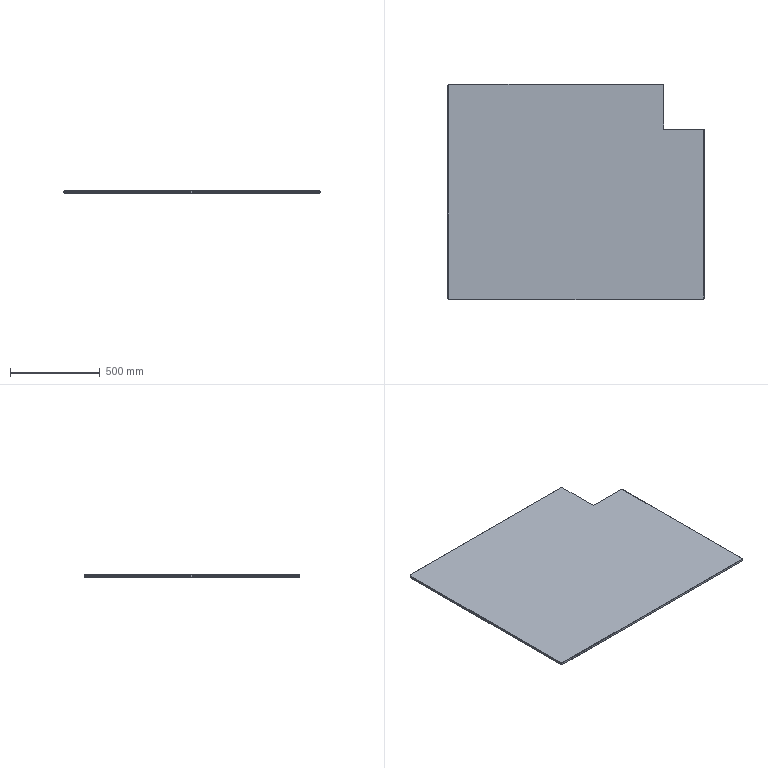Part | STEP file | 1200x1425x13 aluminium plateC-1.STEP | 1 solid | 25 faces | box 1425 x 1200 x 13 mm | volume 21493737 mm3 | plane 16 | cone 6 | cylinder 3 | commonest cylinder face diameters 20 x3
STEP:
#1=CARTESIAN_POINT('',(712.5,350.2,1.));
#2=VERTEX_POINT('',#1);
#3=CARTESIAN_POINT('',(711.5,350.2,0.));
#4=VERTEX_POINT('',#3);
#5=CARTESIAN_POINT('',(712.5,350.2,1.));
#6=DIRECTION('',(-0.7071,0.,-0.7071));
#7=VECTOR('',#6,1000.);
#8=LINE('',#5,#7);
#9=EDGE_CURVE('',#2,#4,#8,.T.);
#10=ORIENTED_EDGE('',*,*,#9,.T.);
#11=CARTESIAN_POINT('',(487.5,350.2,0.));
#12=VERTEX_POINT('',#11);
#13=CARTESIAN_POINT('',(712.5,350.2,0.));
#14=DIRECTION('',(-1.,0.,0.));
#15=VECTOR('',#14,1000.);
#16=LINE('',#13,#15);
#17=EDGE_CURVE('',#4,#12,#16,.T.);
#18=ORIENTED_EDGE('',*,*,#17,.T.);
#19=CARTESIAN_POINT('',(487.5,350.2,13.));
#20=VERTEX_POINT('',#19);
#21=CARTESIAN_POINT('',(487.5,350.2,13.));
#22=DIRECTION('',(0.,0.,-1.));
#23=VECTOR('',#22,1000.);
#24=LINE('',#21,#23);
#25=EDGE_CURVE('',#20,#12,#24,.T.);
#26=ORIENTED_EDGE('',*,*,#25,.F.);
#27=CARTESIAN_POINT('',(711.5,350.2,13.));
#28=VERTEX_POINT('',#27);
#29=CARTESIAN_POINT('',(712.5,350.2,13.));
#30=DIRECTION('',(-1.,0.,0.));
#31=VECTOR('',#30,1000.);
#32=LINE('',#29,#31);
#33=EDGE_CURVE('',#28,#20,#32,.T.);
#34=ORIENTED_EDGE('',*,*,#33,.F.);
#35=CARTESIAN_POINT('',(712.5,350.2,12.));
#36=VERTEX_POINT('',#35);
#37=CARTESIAN_POINT('',(711.5,350.2,13.));
#38=DIRECTION('',(0.7071,0.,-0.7071));
#39=VECTOR('',#38,1000.);
#40=LINE('',#37,#39);
#41=EDGE_CURVE('',#28,#36,#40,.T.);
#42=ORIENTED_EDGE('',*,*,#41,.T.);
#43=CARTESIAN_POINT('',(712.5,350.2,13.));
#44=DIRECTION('',(0.,0.,-1.));
#45=VECTOR('',#44,1000.);
#46=LINE('',#43,#45);
#47=EDGE_CURVE('',#36,#2,#46,.T.);
#48=ORIENTED_EDGE('',*,*,#47,.T.);
#49=EDGE_LOOP('',(#10,#18,#26,#34,#42,#48));
#50=FACE_OUTER_BOUND('',#49,.T.);
#51=CARTESIAN_POINT('',(712.5,350.2,13.));
#52=DIRECTION('',(0.,-1.,0.));
#53=DIRECTION('',(0.,0.,-1.));
#54=AXIS2_PLACEMENT_3D('',#51,#52,#53);
#55=PLANE('',#54);
#56=ADVANCED_FACE('',(#50),#55,.F.);
#57=CARTESIAN_POINT('',(487.5,599.,0.));
#58=VERTEX_POINT('',#57);
#59=CARTESIAN_POINT('',(487.5,600.,1.));
#60=VERTEX_POINT('',#59);
#61=CARTESIAN_POINT('',(487.5,600.,1.));
#62=DIRECTION('',(0.,0.7071,0.7071));
#63=VECTOR('',#62,1000.);
#64=LINE('',#61,#63);
#65=EDGE_CURVE('',#58,#60,#64,.T.);
#66=ORIENTED_EDGE('',*,*,#65,.T.);
#67=CARTESIAN_POINT('',(487.5,600.,12.));
#68=VERTEX_POINT('',#67);
#69=CARTESIAN_POINT('',(487.5,600.,13.));
#70=DIRECTION('',(0.,0.,-1.));
#71=VECTOR('',#70,1000.);
#72=LINE('',#69,#71);
#73=EDGE_CURVE('',#68,#60,#72,.T.);
#74=ORIENTED_EDGE('',*,*,#73,.F.);
#75=CARTESIAN_POINT('',(487.5,599.,13.));
#76=VERTEX_POINT('',#75);
#77=CARTESIAN_POINT('',(487.5,599.,13.));
#78=DIRECTION('',(0.,-0.7071,0.7071));
#79=VECTOR('',#78,1000.);
#80=LINE('',#77,#79);
#81=EDGE_CURVE('',#68,#76,#80,.T.);
#82=ORIENTED_EDGE('',*,*,#81,.T.);
#83=CARTESIAN_POINT('',(487.5,600.,13.));
#84=DIRECTION('',(0.,1.,0.));
#85=VECTOR('',#84,1000.);
#86=LINE('',#83,#85);
#87=EDGE_CURVE('',#20,#76,#86,.T.);
#88=ORIENTED_EDGE('',*,*,#87,.F.);
#89=ORIENTED_EDGE('',*,*,#25,.T.);
#90=CARTESIAN_POINT('',(487.5,600.,0.));
#91=DIRECTION('',(0.,1.,0.));
#92=VECTOR('',#91,1000.);
#93=LINE('',#90,#92);
#94=EDGE_CURVE('',#12,#58,#93,.T.);
#95=ORIENTED_EDGE('',*,*,#94,.T.);
#96=EDGE_LOOP('',(#66,#74,#82,#88,#89,#95));
#97=FACE_OUTER_BOUND('',#96,.T.);
#98=CARTESIAN_POINT('',(487.5,600.,13.));
#99=DIRECTION('',(-1.,0.,0.));
#100=DIRECTION('',(0.,0.,1.));
#101=AXIS2_PLACEMENT_3D('',#98,#99,#100);
#102=PLANE('',#101);
#103=ADVANCED_FACE('',(#97),#102,.F.);
#104=CARTESIAN_POINT('',(-702.5,599.,13.));
#105=VERTEX_POINT('',#104);
#106=CARTESIAN_POINT('',(-702.5,600.,12.));
#107=VERTEX_POINT('',#106);
#108=CARTESIAN_POINT('',(-702.5,599.,13.));
#109=DIRECTION('',(0.,0.7071,-0.7071));
#110=VECTOR('',#109,1000.);
#111=LINE('',#108,#110);
#112=EDGE_CURVE('',#105,#107,#111,.T.);
#113=ORIENTED_EDGE('',*,*,#112,.T.);
#114=CARTESIAN_POINT('',(-712.5,590.,12.));
#115=VERTEX_POINT('',#114);
#116=CARTESIAN_POINT('',(-702.5,590.,12.));
#117=DIRECTION('',(0.,0.,-1.));
#118=DIRECTION('',(1.,0.,0.));
#119=AXIS2_PLACEMENT_3D('',#116,#117,#118);
#120=CIRCLE('',#119,10.);
#121=EDGE_CURVE('',#115,#107,#120,.T.);
#122=ORIENTED_EDGE('',*,*,#121,.F.);
#123=CARTESIAN_POINT('',(-711.5,590.,13.));
#124=VERTEX_POINT('',#123);
#125=CARTESIAN_POINT('',(-712.5,590.,12.));
#126=DIRECTION('',(0.7071,0.,0.7071));
#127=VECTOR('',#126,1000.);
#128=LINE('',#125,#127);
#129=EDGE_CURVE('',#115,#124,#128,.T.);
#130=ORIENTED_EDGE('',*,*,#129,.T.);
#131=CARTESIAN_POINT('',(-702.5,590.,13.));
#132=DIRECTION('',(0.,0.,1.));
#133=DIRECTION('',(1.,0.,0.));
#134=AXIS2_PLACEMENT_3D('',#131,#132,#133);
#135=CIRCLE('',#134,9.);
#136=EDGE_CURVE('',#105,#124,#135,.T.);
#137=ORIENTED_EDGE('',*,*,#136,.F.);
#138=EDGE_LOOP('',(#113,#122,#130,#137));
#139=FACE_OUTER_BOUND('',#138,.T.);
#140=CARTESIAN_POINT('',(-702.5,590.,13.));
#141=DIRECTION('',(0.,0.,-1.));
#142=DIRECTION('',(-1.,0.,0.));
#143=AXIS2_PLACEMENT_3D('',#140,#141,#142);
#144=CONICAL_SURFACE('',#143,9.,0.7854);
#145=ADVANCED_FACE('',(#139),#144,.T.);
#146=CARTESIAN_POINT('',(-712.5,-590.,12.));
#147=VERTEX_POINT('',#146);
#148=CARTESIAN_POINT('',(-711.5,-590.,13.));
#149=VERTEX_POINT('',#148);
#150=CARTESIAN_POINT('',(-712.5,-590.,12.));
#151=DIRECTION('',(0.7071,0.,0.7071));
#152=VECTOR('',#151,1000.);
#153=LINE('',#150,#152);
#154=EDGE_CURVE('',#147,#149,#153,.T.);
#155=ORIENTED_EDGE('',*,*,#154,.T.);
#156=CARTESIAN_POINT('',(-711.5,-590.,13.));
#157=DIRECTION('',(0.,-1.,0.));
#158=VECTOR('',#157,1000.);
#159=LINE('',#156,#158);
#160=EDGE_CURVE('',#124,#149,#159,.T.);
#161=ORIENTED_EDGE('',*,*,#160,.F.);
#162=ORIENTED_EDGE('',*,*,#129,.F.);
#163=CARTESIAN_POINT('',(-712.5,590.,12.));
#164=DIRECTION('',(0.,1.,0.));
#165=VECTOR('',#164,1000.);
#166=LINE('',#163,#165);
#167=EDGE_CURVE('',#147,#115,#166,.T.);
#168=ORIENTED_EDGE('',*,*,#167,.F.);
#169=EDGE_LOOP('',(#155,#161,#162,#168));
#170=FACE_OUTER_BOUND('',#169,.T.);
#171=CARTESIAN_POINT('',(-711.5,0.,13.));
#172=DIRECTION('',(-0.7071,0.,0.7071));
#173=DIRECTION('',(0.,1.,0.));
#174=AXIS2_PLACEMENT_3D('',#171,#172,#173);
#175=PLANE('',#174);
#176=ADVANCED_FACE('',(#170),#175,.T.);
#177=ORIENTED_EDGE('',*,*,#81,.F.);
#178=CARTESIAN_POINT('',(702.5,600.,12.));
#179=DIRECTION('',(1.,0.,0.));
#180=VECTOR('',#179,1000.);
#181=LINE('',#178,#180);
#182=EDGE_CURVE('',#107,#68,#181,.T.);
#183=ORIENTED_EDGE('',*,*,#182,.F.);
#184=ORIENTED_EDGE('',*,*,#112,.F.);
#185=CARTESIAN_POINT('',(-702.5,599.,13.));
#186=DIRECTION('',(-1.,0.,0.));
#187=VECTOR('',#186,1000.);
#188=LINE('',#185,#187);
#189=EDGE_CURVE('',#76,#105,#188,.T.);
#190=ORIENTED_EDGE('',*,*,#189,.F.);
#191=EDGE_LOOP('',(#177,#183,#184,#190));
#192=FACE_OUTER_BOUND('',#191,.T.);
#193=CARTESIAN_POINT('',(0.,599.,13.));
#194=DIRECTION('',(0.,0.7071,0.7071));
#195=DIRECTION('',(1.,0.,0.));
#196=AXIS2_PLACEMENT_3D('',#193,#194,#195);
#197=PLANE('',#196);
#198=ADVANCED_FACE('',(#192),#197,.T.);
#199=CARTESIAN_POINT('',(-702.5,-600.,12.));
#200=VERTEX_POINT('',#199);
#201=CARTESIAN_POINT('',(-702.5,-599.,13.));
#202=VERTEX_POINT('',#201);
#203=CARTESIAN_POINT('',(-702.5,-600.,12.));
#204=DIRECTION('',(0.,0.7071,0.7071));
#205=VECTOR('',#204,1000.);
#206=LINE('',#203,#205);
#207=EDGE_CURVE('',#200,#202,#206,.T.);
#208=ORIENTED_EDGE('',*,*,#207,.T.);
#209=CARTESIAN_POINT('',(-702.5,-590.,13.));
#210=DIRECTION('',(0.,0.,1.));
#211=DIRECTION('',(1.,0.,0.));
#212=AXIS2_PLACEMENT_3D('',#209,#210,#211);
#213=CIRCLE('',#212,9.);
#214=EDGE_CURVE('',#149,#202,#213,.T.);
#215=ORIENTED_EDGE('',*,*,#214,.F.);
#216=ORIENTED_EDGE('',*,*,#154,.F.);
#217=CARTESIAN_POINT('',(-702.5,-590.,12.));
#218=DIRECTION('',(0.,0.,-1.));
#219=DIRECTION('',(1.,0.,0.));
#220=AXIS2_PLACEMENT_3D('',#217,#218,#219);
#221=CIRCLE('',#220,10.);
#222=EDGE_CURVE('',#200,#147,#221,.T.);
#223=ORIENTED_EDGE('',*,*,#222,.F.);
#224=EDGE_LOOP('',(#208,#215,#216,#223));
#225=FACE_OUTER_BOUND('',#224,.T.);
#226=CARTESIAN_POINT('',(-702.5,-590.,13.));
#227=DIRECTION('',(0.,0.,-1.));
#228=DIRECTION('',(-1.,0.,0.));
#229=AXIS2_PLACEMENT_3D('',#226,#227,#228);
#230=CONICAL_SURFACE('',#229,9.,0.7854);
#231=ADVANCED_FACE('',(#225),#230,.T.);
#232=CARTESIAN_POINT('',(702.5,-600.,12.));
#233=VERTEX_POINT('',#232);
#234=CARTESIAN_POINT('',(702.5,-599.,13.));
#235=VERTEX_POINT('',#234);
#236=CARTESIAN_POINT('',(702.5,-600.,12.));
#237=DIRECTION('',(0.,0.7071,0.7071));
#238=VECTOR('',#237,1000.);
#239=LINE('',#236,#238);
#240=EDGE_CURVE('',#233,#235,#239,.T.);
#241=ORIENTED_EDGE('',*,*,#240,.T.);
#242=CARTESIAN_POINT('',(702.5,-599.,13.));
#243=DIRECTION('',(1.,0.,0.));
#244=VECTOR('',#243,1000.);
#245=LINE('',#242,#244);
#246=EDGE_CURVE('',#202,#235,#245,.T.);
#247=ORIENTED_EDGE('',*,*,#246,.F.);
#248=ORIENTED_EDGE('',*,*,#207,.F.);
#249=CARTESIAN_POINT('',(-702.5,-600.,12.));
#250=DIRECTION('',(-1.,0.,0.));
#251=VECTOR('',#250,1000.);
#252=LINE('',#249,#251);
#253=EDGE_CURVE('',#233,#200,#252,.T.);
#254=ORIENTED_EDGE('',*,*,#253,.F.);
#255=EDGE_LOOP('',(#241,#247,#248,#254));
#256=FACE_OUTER_BOUND('',#255,.T.);
#257=CARTESIAN_POINT('',(0.,-599.,13.));
#258=DIRECTION('',(0.,-0.7071,0.7071));
#259=DIRECTION('',(-1.,0.,0.));
#260=AXIS2_PLACEMENT_3D('',#257,#258,#259);
#261=PLANE('',#260);
#262=ADVANCED_FACE('',(#256),#261,.T.);
#263=ORIENTED_EDGE('',*,*,#41,.F.);
#264=CARTESIAN_POINT('',(711.5,-590.,13.));
#265=VERTEX_POINT('',#264);
#266=CARTESIAN_POINT('',(711.5,590.,13.));
#267=DIRECTION('',(0.,1.,0.));
#268=VECTOR('',#267,1000.);
#269=LINE('',#266,#268);
#270=EDGE_CURVE('',#265,#28,#269,.T.);
#271=ORIENTED_EDGE('',*,*,#270,.F.);
#272=CARTESIAN_POINT('',(712.5,-590.,12.));
#273=VERTEX_POINT('',#272);
#274=CARTESIAN_POINT('',(711.5,-590.,13.));
#275=DIRECTION('',(0.7071,0.,-0.7071));
#276=VECTOR('',#275,1000.);
#277=LINE('',#274,#276);
#278=EDGE_CURVE('',#265,#273,#277,.T.);
#279=ORIENTED_EDGE('',*,*,#278,.T.);
#280=CARTESIAN_POINT('',(712.5,-590.,12.));
#281=DIRECTION('',(0.,-1.,0.));
#282=VECTOR('',#281,1000.);
#283=LINE('',#280,#282);
#284=EDGE_CURVE('',#36,#273,#283,.T.);
#285=ORIENTED_EDGE('',*,*,#284,.F.);
#286=EDGE_LOOP('',(#263,#271,#279,#285));
#287=FACE_OUTER_BOUND('',#286,.T.);
#288=CARTESIAN_POINT('',(711.5,0.,13.));
#289=DIRECTION('',(0.7071,0.,0.7071));
#290=DIRECTION('',(0.,-1.,0.));
#291=AXIS2_PLACEMENT_3D('',#288,#289,#290);
#292=PLANE('',#291);
#293=ADVANCED_FACE('',(#287),#292,.T.);
#294=ORIENTED_EDGE('',*,*,#240,.F.);
#295=CARTESIAN_POINT('',(702.5,-590.,12.));
#296=DIRECTION('',(0.,0.,-1.));
#297=DIRECTION('',(1.,0.,0.));
#298=AXIS2_PLACEMENT_3D('',#295,#296,#297);
#299=CIRCLE('',#298,10.);
#300=EDGE_CURVE('',#273,#233,#299,.T.);
#301=ORIENTED_EDGE('',*,*,#300,.F.);
#302=ORIENTED_EDGE('',*,*,#278,.F.);
#303=CARTESIAN_POINT('',(702.5,-590.,13.));
#304=DIRECTION('',(0.,0.,1.));
#305=DIRECTION('',(1.,0.,0.));
#306=AXIS2_PLACEMENT_3D('',#303,#304,#305);
#307=CIRCLE('',#306,9.);
#308=EDGE_CURVE('',#235,#265,#307,.T.);
#309=ORIENTED_EDGE('',*,*,#308,.F.);
#310=EDGE_LOOP('',(#294,#301,#302,#309));
#311=FACE_OUTER_BOUND('',#310,.T.);
#312=CARTESIAN_POINT('',(702.5,-590.,13.));
#313=DIRECTION('',(0.,0.,-1.));
#314=DIRECTION('',(-1.,0.,0.));
#315=AXIS2_PLACEMENT_3D('',#312,#313,#314);
#316=CONICAL_SURFACE('',#315,9.,0.7854);
#317=ADVANCED_FACE('',(#311),#316,.T.);
#318=CARTESIAN_POINT('',(711.5,-590.,0.));
#319=VERTEX_POINT('',#318);
#320=CARTESIAN_POINT('',(712.5,-590.,1.));
#321=VERTEX_POINT('',#320);
#322=CARTESIAN_POINT('',(711.5,-590.,0.));
#323=DIRECTION('',(0.7071,0.,0.7071));
#324=VECTOR('',#323,1000.);
#325=LINE('',#322,#324);
#326=EDGE_CURVE('',#319,#321,#325,.T.);
#327=ORIENTED_EDGE('',*,*,#326,.T.);
#328=CARTESIAN_POINT('',(702.5,-600.,1.));
#329=VERTEX_POINT('',#328);
#330=CARTESIAN_POINT('',(702.5,-590.,1.));
#331=DIRECTION('',(0.,0.,1.));
#332=DIRECTION('',(1.,0.,0.));
#333=AXIS2_PLACEMENT_3D('',#330,#331,#332);
#334=CIRCLE('',#333,10.);
#335=EDGE_CURVE('',#329,#321,#334,.T.);
#336=ORIENTED_EDGE('',*,*,#335,.F.);
#337=CARTESIAN_POINT('',(702.5,-599.,0.));
#338=VERTEX_POINT('',#337);
#339=CARTESIAN_POINT('',(702.5,-600.,1.));
#340=DIRECTION('',(0.,0.7071,-0.7071));
#341=VECTOR('',#340,1000.);
#342=LINE('',#339,#341);
#343=EDGE_CURVE('',#329,#338,#342,.T.);
#344=ORIENTED_EDGE('',*,*,#343,.T.);
#345=CARTESIAN_POINT('',(702.5,-590.,0.));
#346=DIRECTION('',(0.,0.,-1.));
#347=DIRECTION('',(1.,0.,0.));
#348=AXIS2_PLACEMENT_3D('',#345,#346,#347);
#349=CIRCLE('',#348,9.);
#350=EDGE_CURVE('',#319,#338,#349,.T.);
#351=ORIENTED_EDGE('',*,*,#350,.F.);
#352=EDGE_LOOP('',(#327,#336,#344,#351));
#353=FACE_OUTER_BOUND('',#352,.T.);
#354=CARTESIAN_POINT('',(702.5,-590.,0.));
#355=DIRECTION('',(0.,0.,1.));
#356=DIRECTION('',(1.,0.,0.));
#357=AXIS2_PLACEMENT_3D('',#354,#355,#356);
#358=CONICAL_SURFACE('',#357,9.,0.7854);
#359=ADVANCED_FACE('',(#353),#358,.T.);
#360=CARTESIAN_POINT('',(-702.5,-600.,1.));
#361=VERTEX_POINT('',#360);
#362=CARTESIAN_POINT('',(-702.5,-599.,0.));
#363=VERTEX_POINT('',#362);
#364=CARTESIAN_POINT('',(-702.5,-600.,1.));
#365=DIRECTION('',(0.,0.7071,-0.7071));
#366=VECTOR('',#365,1000.);
#367=LINE('',#364,#366);
#368=EDGE_CURVE('',#361,#363,#367,.T.);
#369=ORIENTED_EDGE('',*,*,#368,.T.);
#370=CARTESIAN_POINT('',(0.,-599.,0.));
#371=DIRECTION('',(-1.,0.,0.));
#372=VECTOR('',#371,1000.);
#373=LINE('',#370,#372);
#374=EDGE_CURVE('',#338,#363,#373,.T.);
#375=ORIENTED_EDGE('',*,*,#374,.F.);
#376=ORIENTED_EDGE('',*,*,#343,.F.);
#377=CARTESIAN_POINT('',(-712.5,-600.,1.));
#378=DIRECTION('',(1.,0.,0.));
#379=VECTOR('',#378,1000.);
#380=LINE('',#377,#379);
#381=EDGE_CURVE('',#361,#329,#380,.T.);
#382=ORIENTED_EDGE('',*,*,#381,.F.);
#383=EDGE_LOOP('',(#369,#375,#376,#382));
#384=FACE_OUTER_BOUND('',#383,.T.);
#385=CARTESIAN_POINT('',(-712.5,-600.,1.));
#386=DIRECTION('',(0.,0.7071,0.7071));
#387=DIRECTION('',(1.,0.,0.));
#388=AXIS2_PLACEMENT_3D('',#385,#386,#387);
#389=PLANE('',#388);
#390=ADVANCED_FACE('',(#384),#389,.F.);
#391=ORIENTED_EDGE('',*,*,#9,.F.);
#392=CARTESIAN_POINT('',(712.5,600.,1.));
#393=DIRECTION('',(0.,1.,0.));
#394=VECTOR('',#393,1000.);
#395=LINE('',#392,#394);
#396=EDGE_CURVE('',#321,#2,#395,.T.);
#397=ORIENTED_EDGE('',*,*,#396,.F.);
#398=ORIENTED_EDGE('',*,*,#326,.F.);
#399=CARTESIAN_POINT('',(711.5,0.,0.));
#400=DIRECTION('',(0.,-1.,0.));
#401=VECTOR('',#400,1000.);
#402=LINE('',#399,#401);
#403=EDGE_CURVE('',#4,#319,#402,.T.);
#404=ORIENTED_EDGE('',*,*,#403,.F.);
#405=EDGE_LOOP('',(#391,#397,#398,#404));
#406=FACE_OUTER_BOUND('',#405,.T.);
#407=CARTESIAN_POINT('',(712.5,600.,1.));
#408=DIRECTION('',(-0.7071,0.,0.7071));
#409=DIRECTION('',(0.,1.,0.));
#410=AXIS2_PLACEMENT_3D('',#407,#408,#409);
#411=PLANE('',#410);
#412=ADVANCED_FACE('',(#406),#411,.F.);
#413=CARTESIAN_POINT('',(-712.5,-590.,1.));
#414=VERTEX_POINT('',#413);
#415=CARTESIAN_POINT('',(-711.5,-590.,0.));
#416=VERTEX_POINT('',#415);
#417=CARTESIAN_POINT('',(-712.5,-590.,1.));
#418=DIRECTION('',(0.7071,0.,-0.7071));
#419=VECTOR('',#418,1000.);
#420=LINE('',#417,#419);
#421=EDGE_CURVE('',#414,#416,#420,.T.);
#422=ORIENTED_EDGE('',*,*,#421,.T.);
#423=CARTESIAN_POINT('',(-702.5,-590.,0.));
#424=DIRECTION('',(0.,0.,-1.));
#425=DIRECTION('',(1.,0.,0.));
#426=AXIS2_PLACEMENT_3D('',#423,#424,#425);
#427=CIRCLE('',#426,9.);
#428=EDGE_CURVE('',#363,#416,#427,.T.);
#429=ORIENTED_EDGE('',*,*,#428,.F.);
#430=ORIENTED_EDGE('',*,*,#368,.F.);
#431=CARTESIAN_POINT('',(-702.5,-590.,1.));
#432=DIRECTION('',(0.,0.,1.));
#433=DIRECTION('',(1.,0.,0.));
#434=AXIS2_PLACEMENT_3D('',#431,#432,#433);
#435=CIRCLE('',#434,10.);
#436=EDGE_CURVE('',#414,#361,#435,.T.);
#437=ORIENTED_EDGE('',*,*,#436,.F.);
#438=EDGE_LOOP('',(#422,#429,#430,#437));
#439=FACE_OUTER_BOUND('',#438,.T.);
#440=CARTESIAN_POINT('',(-702.5,-590.,0.));
#441=DIRECTION('',(0.,0.,1.));
#442=DIRECTION('',(1.,0.,0.));
#443=AXIS2_PLACEMENT_3D('',#440,#441,#442);
#444=CONICAL_SURFACE('',#443,9.,0.7854);
#445=ADVANCED_FACE('',(#439),#444,.T.);
#446=CARTESIAN_POINT('',(-712.5,590.,1.));
#447=VERTEX_POINT('',#446);
#448=CARTESIAN_POINT('',(-711.5,590.,0.));
#449=VERTEX_POINT('',#448);
#450=CARTESIAN_POINT('',(-712.5,590.,1.));
#451=DIRECTION('',(0.7071,0.,-0.7071));
#452=VECTOR('',#451,1000.);
#453=LINE('',#450,#452);
#454=EDGE_CURVE('',#447,#449,#453,.T.);
#455=ORIENTED_EDGE('',*,*,#454,.T.);
#456=CARTESIAN_POINT('',(-711.5,0.,0.));
#457=DIRECTION('',(0.,1.,0.));
#458=VECTOR('',#457,1000.);
#459=LINE('',#456,#458);
#460=EDGE_CURVE('',#416,#449,#459,.T.);
#461=ORIENTED_EDGE('',*,*,#460,.F.);
#462=ORIENTED_EDGE('',*,*,#421,.F.);
#463=CARTESIAN_POINT('',(-712.5,600.,1.));
#464=DIRECTION('',(0.,-1.,0.));
#465=VECTOR('',#464,1000.);
#466=LINE('',#463,#465);
#467=EDGE_CURVE('',#447,#414,#466,.T.);
#468=ORIENTED_EDGE('',*,*,#467,.F.);
#469=EDGE_LOOP('',(#455,#461,#462,#468));
#470=FACE_OUTER_BOUND('',#469,.T.);
#471=CARTESIAN_POINT('',(-712.5,600.,1.));
#472=DIRECTION('',(0.7071,0.,0.7071));
#473=DIRECTION('',(0.,-1.,0.));
#474=AXIS2_PLACEMENT_3D('',#471,#472,#473);
#475=PLANE('',#474);
#476=ADVANCED_FACE('',(#470),#475,.F.);
#477=ORIENTED_EDGE('',*,*,#65,.F.);
#478=CARTESIAN_POINT('',(-702.5,599.,0.));
#479=VERTEX_POINT('',#478);
#480=CARTESIAN_POINT('',(0.,599.,0.));
#481=DIRECTION('',(1.,0.,0.));
#482=VECTOR('',#481,1000.);
#483=LINE('',#480,#482);
#484=EDGE_CURVE('',#479,#58,#483,.T.);
#485=ORIENTED_EDGE('',*,*,#484,.F.);
#486=CARTESIAN_POINT('',(-702.5,600.,1.));
#487=VERTEX_POINT('',#486);
#488=CARTESIAN_POINT('',(-702.5,599.,0.));
#489=DIRECTION('',(0.,0.7071,0.7071));
#490=VECTOR('',#489,1000.);
#491=LINE('',#488,#490);
#492=EDGE_CURVE('',#479,#487,#491,.T.);
#493=ORIENTED_EDGE('',*,*,#492,.T.);
#494=CARTESIAN_POINT('',(-712.5,600.,1.));
#495=DIRECTION('',(-1.,0.,0.));
#496=VECTOR('',#495,1000.);
#497=LINE('',#494,#496);
#498=EDGE_CURVE('',#60,#487,#497,.T.);
#499=ORIENTED_EDGE('',*,*,#498,.F.);
#500=EDGE_LOOP('',(#477,#485,#493,#499));
#501=FACE_OUTER_BOUND('',#500,.T.);
#502=CARTESIAN_POINT('',(-712.5,600.,1.));
#503=DIRECTION('',(0.,-0.7071,0.7071));
#504=DIRECTION('',(-1.,0.,0.));
#505=AXIS2_PLACEMENT_3D('',#502,#503,#504);
#506=PLANE('',#505);
#507=ADVANCED_FACE('',(#501),#506,.F.);
#508=ORIENTED_EDGE('',*,*,#454,.F.);
#509=CARTESIAN_POINT('',(-702.5,590.,1.));
#510=DIRECTION('',(0.,0.,1.));
#511=DIRECTION('',(1.,0.,0.));
#512=AXIS2_PLACEMENT_3D('',#509,#510,#511);
#513=CIRCLE('',#512,10.);
#514=EDGE_CURVE('',#487,#447,#513,.T.);
#515=ORIENTED_EDGE('',*,*,#514,.F.);
#516=ORIENTED_EDGE('',*,*,#492,.F.);
#517=CARTESIAN_POINT('',(-702.5,590.,0.));
#518=DIRECTION('',(0.,0.,-1.));
#519=DIRECTION('',(1.,0.,0.));
#520=AXIS2_PLACEMENT_3D('',#517,#518,#519);
#521=CIRCLE('',#520,9.);
#522=EDGE_CURVE('',#449,#479,#521,.T.);
#523=ORIENTED_EDGE('',*,*,#522,.F.);
#524=EDGE_LOOP('',(#508,#515,#516,#523));
#525=FACE_OUTER_BOUND('',#524,.T.);
#526=CARTESIAN_POINT('',(-702.5,590.,0.));
#527=DIRECTION('',(0.,0.,1.));
#528=DIRECTION('',(1.,0.,0.));
#529=AXIS2_PLACEMENT_3D('',#526,#527,#528);
#530=CONICAL_SURFACE('',#529,9.,0.7854);
#531=ADVANCED_FACE('',(#525),#530,.T.);
#532=CARTESIAN_POINT('',(-702.5,600.,13.));
#533=DIRECTION('',(0.,0.,1.));
#534=VECTOR('',#533,1000.);
#535=LINE('',#532,#534);
#536=EDGE_CURVE('',#487,#107,#535,.T.);
#537=ORIENTED_EDGE('',*,*,#536,.F.);
#538=ORIENTED_EDGE('',*,*,#514,.T.);
#539=CARTESIAN_POINT('',(-712.5,590.,13.));
#540=DIRECTION('',(0.,0.,-1.));
#541=VECTOR('',#540,1000.);
#542=LINE('',#539,#541);
#543=EDGE_CURVE('',#115,#447,#542,.T.);
#544=ORIENTED_EDGE('',*,*,#543,.F.);
#545=ORIENTED_EDGE('',*,*,#121,.T.);
#546=EDGE_LOOP('',(#537,#538,#544,#545));
#547=FACE_OUTER_BOUND('',#546,.T.);
#548=CARTESIAN_POINT('',(-702.5,590.,13.));
#549=DIRECTION('',(0.,0.,-1.));
#550=DIRECTION('',(-1.,0.,0.));
#551=AXIS2_PLACEMENT_3D('',#548,#549,#550);
#552=CYLINDRICAL_SURFACE('',#551,10.);
#553=ADVANCED_FACE('',(#547),#552,.T.);
#554=CARTESIAN_POINT('',(702.5,-600.,13.));
#555=DIRECTION('',(0.,0.,1.));
#556=VECTOR('',#555,1000.);
#557=LINE('',#554,#556);
#558=EDGE_CURVE('',#329,#233,#557,.T.);
#559=ORIENTED_EDGE('',*,*,#558,.F.);
#560=ORIENTED_EDGE('',*,*,#335,.T.);
#561=CARTESIAN_POINT('',(712.5,-590.,13.));
#562=DIRECTION('',(0.,0.,-1.));
#563=VECTOR('',#562,1000.);
#564=LINE('',#561,#563);
#565=EDGE_CURVE('',#273,#321,#564,.T.);
#566=ORIENTED_EDGE('',*,*,#565,.F.);
#567=ORIENTED_EDGE('',*,*,#300,.T.);
#568=EDGE_LOOP('',(#559,#560,#566,#567));
#569=FACE_OUTER_BOUND('',#568,.T.);
#570=CARTESIAN_POINT('',(702.5,-590.,13.));
#571=DIRECTION('',(0.,0.,-1.));
#572=DIRECTION('',(-1.,0.,0.));
#573=AXIS2_PLACEMENT_3D('',#570,#571,#572);
#574=CYLINDRICAL_SURFACE('',#573,10.);
#575=ADVANCED_FACE('',(#569),#574,.T.);
#576=CARTESIAN_POINT('',(-712.5,-590.,13.));
#577=DIRECTION('',(0.,0.,1.));
#578=VECTOR('',#577,1000.);
#579=LINE('',#576,#578);
#580=EDGE_CURVE('',#414,#147,#579,.T.);
#581=ORIENTED_EDGE('',*,*,#580,.F.);
#582=ORIENTED_EDGE('',*,*,#436,.T.);
#583=CARTESIAN_POINT('',(-702.5,-600.,13.));
#584=DIRECTION('',(0.,0.,-1.));
#585=VECTOR('',#584,1000.);
#586=LINE('',#583,#585);
#587=EDGE_CURVE('',#200,#361,#586,.T.);
#588=ORIENTED_EDGE('',*,*,#587,.F.);
#589=ORIENTED_EDGE('',*,*,#222,.T.);
#590=EDGE_LOOP('',(#581,#582,#588,#589));
#591=FACE_OUTER_BOUND('',#590,.T.);
#592=CARTESIAN_POINT('',(-702.5,-590.,13.));
#593=DIRECTION('',(0.,0.,-1.));
#594=DIRECTION('',(-1.,0.,0.));
#595=AXIS2_PLACEMENT_3D('',#592,#593,#594);
#596=CYLINDRICAL_SURFACE('',#595,10.);
#597=ADVANCED_FACE('',(#591),#596,.T.);
#598=ORIENTED_EDGE('',*,*,#484,.T.);
#599=ORIENTED_EDGE('',*,*,#94,.F.);
#600=ORIENTED_EDGE('',*,*,#17,.F.);
#601=ORIENTED_EDGE('',*,*,#403,.T.);
#602=ORIENTED_EDGE('',*,*,#350,.T.);
#603=ORIENTED_EDGE('',*,*,#374,.T.);
#604=ORIENTED_EDGE('',*,*,#428,.T.);
#605=ORIENTED_EDGE('',*,*,#460,.T.);
#606=ORIENTED_EDGE('',*,*,#522,.T.);
#607=EDGE_LOOP('',(#598,#599,#600,#601,#602,#603,#604,#605,#606));
#608=FACE_OUTER_BOUND('',#607,.T.);
#609=CARTESIAN_POINT('',(0.,0.,0.));
#610=DIRECTION('',(0.,0.,1.));
#611=DIRECTION('',(1.,0.,0.));
#612=AXIS2_PLACEMENT_3D('',#609,#610,#611);
#613=PLANE('',#612);
#614=ADVANCED_FACE('',(#608),#613,.F.);
#615=ORIENTED_EDGE('',*,*,#87,.T.);
#616=ORIENTED_EDGE('',*,*,#189,.T.);
#617=ORIENTED_EDGE('',*,*,#136,.T.);
#618=ORIENTED_EDGE('',*,*,#160,.T.);
#619=ORIENTED_EDGE('',*,*,#214,.T.);
#620=ORIENTED_EDGE('',*,*,#246,.T.);
#621=ORIENTED_EDGE('',*,*,#308,.T.);
#622=ORIENTED_EDGE('',*,*,#270,.T.);
#623=ORIENTED_EDGE('',*,*,#33,.T.);
#624=EDGE_LOOP('',(#615,#616,#617,#618,#619,#620,#621,#622,#623));
#625=FACE_OUTER_BOUND('',#624,.T.);
#626=CARTESIAN_POINT('',(0.,0.,13.));
#627=DIRECTION('',(0.,0.,1.));
#628=DIRECTION('',(1.,0.,0.));
#629=AXIS2_PLACEMENT_3D('',#626,#627,#628);
#630=PLANE('',#629);
#631=ADVANCED_FACE('',(#625),#630,.T.);
#632=ORIENTED_EDGE('',*,*,#587,.T.);
#633=ORIENTED_EDGE('',*,*,#381,.T.);
#634=ORIENTED_EDGE('',*,*,#558,.T.);
#635=ORIENTED_EDGE('',*,*,#253,.T.);
#636=EDGE_LOOP('',(#632,#633,#634,#635));
#637=FACE_OUTER_BOUND('',#636,.T.);
#638=CARTESIAN_POINT('',(-712.5,-600.,13.));
#639=DIRECTION('',(0.,1.,0.));
#640=DIRECTION('',(1.,0.,0.));
#641=AXIS2_PLACEMENT_3D('',#638,#639,#640);
#642=PLANE('',#641);
#643=ADVANCED_FACE('',(#637),#642,.F.);
#644=ORIENTED_EDGE('',*,*,#543,.T.);
#645=ORIENTED_EDGE('',*,*,#467,.T.);
#646=ORIENTED_EDGE('',*,*,#580,.T.);
#647=ORIENTED_EDGE('',*,*,#167,.T.);
#648=EDGE_LOOP('',(#644,#645,#646,#647));
#649=FACE_OUTER_BOUND('',#648,.T.);
#650=CARTESIAN_POINT('',(-712.5,600.,13.));
#651=DIRECTION('',(1.,0.,0.));
#652=DIRECTION('',(0.,1.,0.));
#653=AXIS2_PLACEMENT_3D('',#650,#651,#652);
#654=PLANE('',#653);
#655=ADVANCED_FACE('',(#649),#654,.F.);
#656=ORIENTED_EDGE('',*,*,#182,.T.);
#657=ORIENTED_EDGE('',*,*,#73,.T.);
#658=ORIENTED_EDGE('',*,*,#498,.T.);
#659=ORIENTED_EDGE('',*,*,#536,.T.);
#660=EDGE_LOOP('',(#656,#657,#658,#659));
#661=FACE_OUTER_BOUND('',#660,.T.);
#662=CARTESIAN_POINT('',(-712.5,600.,13.));
#663=DIRECTION('',(0.,-1.,0.));
#664=DIRECTION('',(0.,0.,-1.));
#665=AXIS2_PLACEMENT_3D('',#662,#663,#664);
#666=PLANE('',#665);
#667=ADVANCED_FACE('',(#661),#666,.F.);
#668=ORIENTED_EDGE('',*,*,#396,.T.);
#669=ORIENTED_EDGE('',*,*,#47,.F.);
#670=ORIENTED_EDGE('',*,*,#284,.T.);
#671=ORIENTED_EDGE('',*,*,#565,.T.);
#672=EDGE_LOOP('',(#668,#669,#670,#671));
#673=FACE_OUTER_BOUND('',#672,.T.);
#674=CARTESIAN_POINT('',(712.5,600.,13.));
#675=DIRECTION('',(-1.,0.,0.));
#676=DIRECTION('',(0.,1.,0.));
#677=AXIS2_PLACEMENT_3D('',#674,#675,#676);
#678=PLANE('',#677);
#679=ADVANCED_FACE('',(#673),#678,.F.);
#680=CLOSED_SHELL('',(#56,#103,#145,#176,#198,#231,#262,#293,#317,#359,#390,#412,#445,#476,#507,#531,#553,#575,#597,#614,#631,#643,#655,#667,#679));
#681=MANIFOLD_SOLID_BREP('',#680);
#682=CARTESIAN_POINT('',(0.,0.,0.));
#683=DIRECTION('',(0.,0.,1.));
#684=DIRECTION('',(1.,0.,0.));
#685=AXIS2_PLACEMENT_3D('',#682,#683,#684);
#686=(LENGTH_UNIT()NAMED_UNIT(*)SI_UNIT(.MILLI.,.METRE.));
#687=UNCERTAINTY_MEASURE_WITH_UNIT(LENGTH_MEASURE(0.00001),#686,'','');
#688=(NAMED_UNIT(*)PLANE_ANGLE_UNIT()SI_UNIT($,.RADIAN.));
#689=(NAMED_UNIT(*)SI_UNIT($,.STERADIAN.)SOLID_ANGLE_UNIT());
#690=(GEOMETRIC_REPRESENTATION_CONTEXT(3)GLOBAL_UNCERTAINTY_ASSIGNED_CONTEXT((#687))GLOBAL_UNIT_ASSIGNED_CONTEXT((#686,#688,#689))REPRESENTATION_CONTEXT('',''));
#691=ADVANCED_BREP_SHAPE_REPRESENTATION('',(#681,#685),#690);